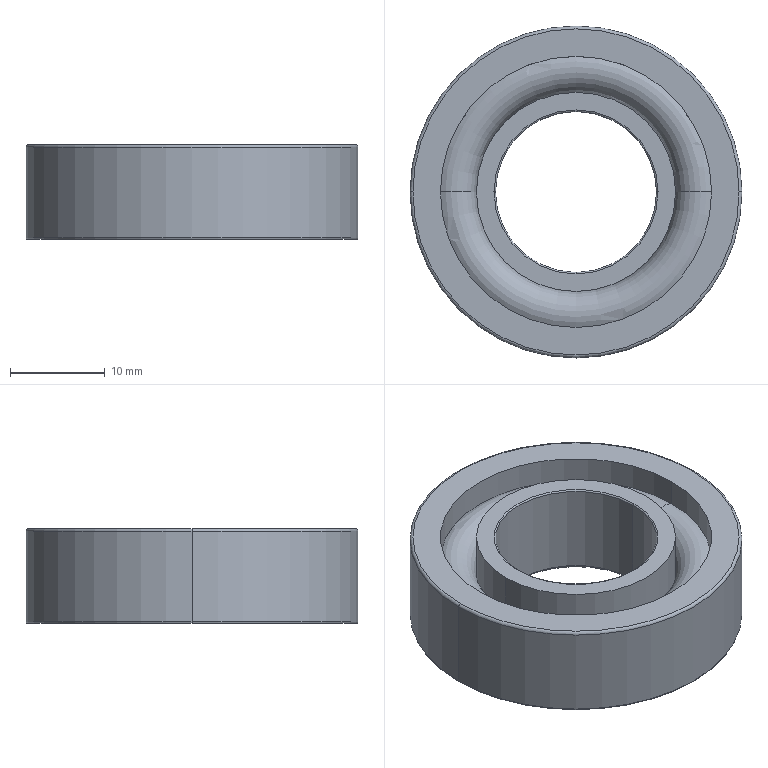Part | SolidWorks | features BaseBody 1 | 1 solid | 28 faces | box 35 x 35 x 10 mm | volume 5588 mm3 | torus 12 | cylinder 12 | plane 4 | commonest cylinder face diameters 17 x2 21 x2 23.75 x2 28.6 x2 31 x2 35 x2
STEP:
#1=CARTESIAN_POINT('',(-17.5,0.,-9.85));
#2=VERTEX_POINT('',#1);
#3=CARTESIAN_POINT('',(17.5,0.,-9.85));
#4=VERTEX_POINT('',#3);
#5=CARTESIAN_POINT('',(0.,0.,-9.85));
#6=DIRECTION('',(0.,0.,-1.));
#7=DIRECTION('',(-1.,0.,0.));
#8=AXIS2_PLACEMENT_3D('',#5,#6,#7);
#9=CIRCLE('',#8,17.5);
#10=EDGE_CURVE('',#2,#4,#9,.T.);
#11=ORIENTED_EDGE('',*,*,#10,.T.);
#12=CARTESIAN_POINT('',(17.35,0.,-10.));
#13=VERTEX_POINT('',#12);
#14=CARTESIAN_POINT('',(17.35,0.,-9.85));
#15=DIRECTION('',(0.,1.,0.));
#16=DIRECTION('',(-1.,0.,0.));
#17=AXIS2_PLACEMENT_3D('',#14,#15,#16);
#18=CIRCLE('',#17,0.15);
#19=EDGE_CURVE('',#4,#13,#18,.T.);
#20=ORIENTED_EDGE('',*,*,#19,.T.);
#21=CARTESIAN_POINT('',(-17.35,0.,-10.));
#22=VERTEX_POINT('',#21);
#23=CARTESIAN_POINT('',(0.,0.,-10.));
#24=DIRECTION('',(0.,0.,-1.));
#25=DIRECTION('',(-1.,0.,0.));
#26=AXIS2_PLACEMENT_3D('',#23,#24,#25);
#27=CIRCLE('',#26,17.35);
#28=EDGE_CURVE('',#22,#13,#27,.T.);
#29=ORIENTED_EDGE('',*,*,#28,.F.);
#30=CARTESIAN_POINT('',(-17.35,0.,-9.85));
#31=DIRECTION('',(0.,-1.,0.));
#32=DIRECTION('',(0.,0.,-1.));
#33=AXIS2_PLACEMENT_3D('',#30,#31,#32);
#34=CIRCLE('',#33,0.15);
#35=EDGE_CURVE('',#2,#22,#34,.T.);
#36=ORIENTED_EDGE('',*,*,#35,.F.);
#37=EDGE_LOOP('',(#11,#20,#29,#36));
#38=FACE_OUTER_BOUND('',#37,.T.);
#39=CARTESIAN_POINT('',(0.,0.,-9.85));
#40=DIRECTION('',(0.,0.,-1.));
#41=DIRECTION('',(-1.,0.,0.));
#42=AXIS2_PLACEMENT_3D('',#39,#40,#41);
#43=TOROIDAL_SURFACE('',#42,17.35,0.15);
#44=ADVANCED_FACE('',(#38),#43,.T.);
#45=CARTESIAN_POINT('',(15.5,0.,-5.));
#46=VERTEX_POINT('',#45);
#47=CARTESIAN_POINT('',(-15.5,0.,-5.));
#48=VERTEX_POINT('',#47);
#49=CARTESIAN_POINT('',(0.,0.,-5.));
#50=DIRECTION('',(0.,0.,-1.));
#51=DIRECTION('',(-1.,0.,0.));
#52=AXIS2_PLACEMENT_3D('',#49,#50,#51);
#53=CIRCLE('',#52,15.5);
#54=EDGE_CURVE('',#46,#48,#53,.T.);
#55=ORIENTED_EDGE('',*,*,#54,.F.);
#56=CARTESIAN_POINT('',(15.5,0.,-10.));
#57=VERTEX_POINT('',#56);
#58=CARTESIAN_POINT('',(15.5,0.,-10.));
#59=DIRECTION('',(0.,0.,-1.));
#60=VECTOR('',#59,1000.);
#61=LINE('',#58,#60);
#62=EDGE_CURVE('',#46,#57,#61,.T.);
#63=ORIENTED_EDGE('',*,*,#62,.T.);
#64=CARTESIAN_POINT('',(-15.5,0.,-10.));
#65=VERTEX_POINT('',#64);
#66=CARTESIAN_POINT('',(0.,0.,-10.));
#67=DIRECTION('',(0.,0.,-1.));
#68=DIRECTION('',(-1.,0.,0.));
#69=AXIS2_PLACEMENT_3D('',#66,#67,#68);
#70=CIRCLE('',#69,15.5);
#71=EDGE_CURVE('',#57,#65,#70,.T.);
#72=ORIENTED_EDGE('',*,*,#71,.T.);
#73=CARTESIAN_POINT('',(-15.5,0.,-10.));
#74=DIRECTION('',(0.,0.,-1.));
#75=VECTOR('',#74,1000.);
#76=LINE('',#73,#75);
#77=EDGE_CURVE('',#48,#65,#76,.T.);
#78=ORIENTED_EDGE('',*,*,#77,.F.);
#79=EDGE_LOOP('',(#55,#63,#72,#78));
#80=FACE_OUTER_BOUND('',#79,.T.);
#81=CARTESIAN_POINT('',(0.,0.,-10.));
#82=DIRECTION('',(0.,0.,-1.));
#83=DIRECTION('',(-1.,0.,0.));
#84=AXIS2_PLACEMENT_3D('',#81,#82,#83);
#85=CYLINDRICAL_SURFACE('',#84,15.5);
#86=ADVANCED_FACE('',(#80),#85,.F.);
#87=CARTESIAN_POINT('',(-17.5,0.,-0.3));
#88=VERTEX_POINT('',#87);
#89=CARTESIAN_POINT('',(17.5,0.,-0.3));
#90=VERTEX_POINT('',#89);
#91=CARTESIAN_POINT('',(0.,0.,-0.3));
#92=DIRECTION('',(0.,0.,-1.));
#93=DIRECTION('',(-1.,0.,0.));
#94=AXIS2_PLACEMENT_3D('',#91,#92,#93);
#95=CIRCLE('',#94,17.5);
#96=EDGE_CURVE('',#88,#90,#95,.T.);
#97=ORIENTED_EDGE('',*,*,#96,.T.);
#98=CARTESIAN_POINT('',(17.5,0.,-10.));
#99=DIRECTION('',(0.,0.,-1.));
#100=VECTOR('',#99,1000.);
#101=LINE('',#98,#100);
#102=EDGE_CURVE('',#90,#4,#101,.T.);
#103=ORIENTED_EDGE('',*,*,#102,.T.);
#104=ORIENTED_EDGE('',*,*,#10,.F.);
#105=CARTESIAN_POINT('',(-17.5,0.,-10.));
#106=DIRECTION('',(0.,0.,-1.));
#107=VECTOR('',#106,1000.);
#108=LINE('',#105,#107);
#109=EDGE_CURVE('',#88,#2,#108,.T.);
#110=ORIENTED_EDGE('',*,*,#109,.F.);
#111=EDGE_LOOP('',(#97,#103,#104,#110));
#112=FACE_OUTER_BOUND('',#111,.T.);
#113=CARTESIAN_POINT('',(0.,0.,-10.));
#114=DIRECTION('',(0.,0.,-1.));
#115=DIRECTION('',(-1.,0.,0.));
#116=AXIS2_PLACEMENT_3D('',#113,#114,#115);
#117=CYLINDRICAL_SURFACE('',#116,17.5);
#118=ADVANCED_FACE('',(#112),#117,.T.);
#119=CARTESIAN_POINT('',(0.,0.,-5.));
#120=DIRECTION('',(0.,0.,-1.));
#121=DIRECTION('',(-1.,0.,0.));
#122=AXIS2_PLACEMENT_3D('',#119,#120,#121);
#123=CIRCLE('',#122,15.5);
#124=EDGE_CURVE('',#48,#46,#123,.T.);
#125=ORIENTED_EDGE('',*,*,#124,.T.);
#126=CARTESIAN_POINT('',(11.875,0.,-7.233));
#127=VERTEX_POINT('',#126);
#128=CARTESIAN_POINT('',(13.,0.,-5.));
#129=DIRECTION('',(0.,1.,0.));
#130=DIRECTION('',(-1.,0.,0.));
#131=AXIS2_PLACEMENT_3D('',#128,#129,#130);
#132=CIRCLE('',#131,2.5);
#133=EDGE_CURVE('',#46,#127,#132,.T.);
#134=ORIENTED_EDGE('',*,*,#133,.T.);
#135=CARTESIAN_POINT('',(-11.875,0.,-7.233));
#136=VERTEX_POINT('',#135);
#137=CARTESIAN_POINT('',(0.,0.,-7.233));
#138=DIRECTION('',(0.,0.,-1.));
#139=DIRECTION('',(-1.,0.,0.));
#140=AXIS2_PLACEMENT_3D('',#137,#138,#139);
#141=CIRCLE('',#140,11.875);
#142=EDGE_CURVE('',#136,#127,#141,.T.);
#143=ORIENTED_EDGE('',*,*,#142,.F.);
#144=CARTESIAN_POINT('',(-13.,0.,-5.));
#145=DIRECTION('',(0.,-1.,0.));
#146=DIRECTION('',(0.,0.,-1.));
#147=AXIS2_PLACEMENT_3D('',#144,#145,#146);
#148=CIRCLE('',#147,2.5);
#149=EDGE_CURVE('',#48,#136,#148,.T.);
#150=ORIENTED_EDGE('',*,*,#149,.F.);
#151=EDGE_LOOP('',(#125,#134,#143,#150));
#152=FACE_OUTER_BOUND('',#151,.T.);
#153=CARTESIAN_POINT('',(0.,0.,-5.));
#154=DIRECTION('',(0.,0.,-1.));
#155=DIRECTION('',(-1.,0.,0.));
#156=AXIS2_PLACEMENT_3D('',#153,#154,#155);
#157=TOROIDAL_SURFACE('',#156,13.,2.5);
#158=ADVANCED_FACE('',(#152),#157,.T.);
#159=CARTESIAN_POINT('',(-17.2,0.,0.));
#160=VERTEX_POINT('',#159);
#161=CARTESIAN_POINT('',(17.2,0.,0.));
#162=VERTEX_POINT('',#161);
#163=CARTESIAN_POINT('',(0.,0.,0.));
#164=DIRECTION('',(0.,0.,-1.));
#165=DIRECTION('',(-1.,0.,0.));
#166=AXIS2_PLACEMENT_3D('',#163,#164,#165);
#167=CIRCLE('',#166,17.2);
#168=EDGE_CURVE('',#160,#162,#167,.T.);
#169=ORIENTED_EDGE('',*,*,#168,.T.);
#170=CARTESIAN_POINT('',(17.2,0.,-0.3));
#171=DIRECTION('',(0.,1.,0.));
#172=DIRECTION('',(-1.,0.,0.));
#173=AXIS2_PLACEMENT_3D('',#170,#171,#172);
#174=CIRCLE('',#173,0.3);
#175=EDGE_CURVE('',#162,#90,#174,.T.);
#176=ORIENTED_EDGE('',*,*,#175,.T.);
#177=ORIENTED_EDGE('',*,*,#96,.F.);
#178=CARTESIAN_POINT('',(-17.2,0.,-0.3));
#179=DIRECTION('',(0.,-1.,0.));
#180=DIRECTION('',(0.,0.,-1.));
#181=AXIS2_PLACEMENT_3D('',#178,#179,#180);
#182=CIRCLE('',#181,0.3);
#183=EDGE_CURVE('',#160,#88,#182,.T.);
#184=ORIENTED_EDGE('',*,*,#183,.F.);
#185=EDGE_LOOP('',(#169,#176,#177,#184));
#186=FACE_OUTER_BOUND('',#185,.T.);
#187=CARTESIAN_POINT('',(0.,0.,-0.3));
#188=DIRECTION('',(0.,0.,-1.));
#189=DIRECTION('',(-1.,0.,0.));
#190=AXIS2_PLACEMENT_3D('',#187,#188,#189);
#191=TOROIDAL_SURFACE('',#190,17.2,0.3);
#192=ADVANCED_FACE('',(#186),#191,.T.);
#193=ORIENTED_EDGE('',*,*,#142,.T.);
#194=CARTESIAN_POINT('',(11.875,0.,-10.));
#195=VERTEX_POINT('',#194);
#196=CARTESIAN_POINT('',(11.875,0.,-10.));
#197=DIRECTION('',(0.,0.,-1.));
#198=VECTOR('',#197,1000.);
#199=LINE('',#196,#198);
#200=EDGE_CURVE('',#127,#195,#199,.T.);
#201=ORIENTED_EDGE('',*,*,#200,.T.);
#202=CARTESIAN_POINT('',(-11.875,0.,-10.));
#203=VERTEX_POINT('',#202);
#204=CARTESIAN_POINT('',(0.,0.,-10.));
#205=DIRECTION('',(0.,0.,-1.));
#206=DIRECTION('',(-1.,0.,0.));
#207=AXIS2_PLACEMENT_3D('',#204,#205,#206);
#208=CIRCLE('',#207,11.875);
#209=EDGE_CURVE('',#203,#195,#208,.T.);
#210=ORIENTED_EDGE('',*,*,#209,.F.);
#211=CARTESIAN_POINT('',(-11.875,0.,-10.));
#212=DIRECTION('',(0.,0.,-1.));
#213=VECTOR('',#212,1000.);
#214=LINE('',#211,#213);
#215=EDGE_CURVE('',#136,#203,#214,.T.);
#216=ORIENTED_EDGE('',*,*,#215,.F.);
#217=EDGE_LOOP('',(#193,#201,#210,#216));
#218=FACE_OUTER_BOUND('',#217,.T.);
#219=CARTESIAN_POINT('',(0.,0.,-10.));
#220=DIRECTION('',(0.,0.,-1.));
#221=DIRECTION('',(-1.,0.,0.));
#222=AXIS2_PLACEMENT_3D('',#219,#220,#221);
#223=CYLINDRICAL_SURFACE('',#222,11.875);
#224=ADVANCED_FACE('',(#218),#223,.T.);
#225=CARTESIAN_POINT('',(14.3,0.,0.));
#226=VERTEX_POINT('',#225);
#227=CARTESIAN_POINT('',(-14.3,0.,0.));
#228=VERTEX_POINT('',#227);
#229=CARTESIAN_POINT('',(0.,0.,0.));
#230=DIRECTION('',(0.,0.,-1.));
#231=DIRECTION('',(-1.,0.,0.));
#232=AXIS2_PLACEMENT_3D('',#229,#230,#231);
#233=CIRCLE('',#232,14.3);
#234=EDGE_CURVE('',#226,#228,#233,.T.);
#235=ORIENTED_EDGE('',*,*,#234,.F.);
#236=CARTESIAN_POINT('',(14.3,0.,-2.865));
#237=VERTEX_POINT('',#236);
#238=CARTESIAN_POINT('',(14.3,0.,-10.));
#239=DIRECTION('',(0.,0.,-1.));
#240=VECTOR('',#239,1000.);
#241=LINE('',#238,#240);
#242=EDGE_CURVE('',#226,#237,#241,.T.);
#243=ORIENTED_EDGE('',*,*,#242,.T.);
#244=CARTESIAN_POINT('',(-14.3,0.,-2.865));
#245=VERTEX_POINT('',#244);
#246=CARTESIAN_POINT('',(0.,0.,-2.865));
#247=DIRECTION('',(0.,0.,-1.));
#248=DIRECTION('',(-1.,0.,0.));
#249=AXIS2_PLACEMENT_3D('',#246,#247,#248);
#250=CIRCLE('',#249,14.3);
#251=EDGE_CURVE('',#237,#245,#250,.T.);
#252=ORIENTED_EDGE('',*,*,#251,.T.);
#253=CARTESIAN_POINT('',(-14.3,0.,-10.));
#254=DIRECTION('',(0.,0.,-1.));
#255=VECTOR('',#254,1000.);
#256=LINE('',#253,#255);
#257=EDGE_CURVE('',#228,#245,#256,.T.);
#258=ORIENTED_EDGE('',*,*,#257,.F.);
#259=EDGE_LOOP('',(#235,#243,#252,#258));
#260=FACE_OUTER_BOUND('',#259,.T.);
#261=CARTESIAN_POINT('',(0.,0.,-10.));
#262=DIRECTION('',(0.,0.,-1.));
#263=DIRECTION('',(-1.,0.,0.));
#264=AXIS2_PLACEMENT_3D('',#261,#262,#263);
#265=CYLINDRICAL_SURFACE('',#264,14.3);
#266=ADVANCED_FACE('',(#260),#265,.F.);
#267=CARTESIAN_POINT('',(-8.8,0.,-10.));
#268=VERTEX_POINT('',#267);
#269=CARTESIAN_POINT('',(8.8,0.,-10.));
#270=VERTEX_POINT('',#269);
#271=CARTESIAN_POINT('',(0.,0.,-10.));
#272=DIRECTION('',(0.,0.,-1.));
#273=DIRECTION('',(-1.,0.,0.));
#274=AXIS2_PLACEMENT_3D('',#271,#272,#273);
#275=CIRCLE('',#274,8.8);
#276=EDGE_CURVE('',#268,#270,#275,.T.);
#277=ORIENTED_EDGE('',*,*,#276,.T.);
#278=CARTESIAN_POINT('',(8.5,0.,-9.7));
#279=VERTEX_POINT('',#278);
#280=CARTESIAN_POINT('',(8.8,0.,-9.7));
#281=DIRECTION('',(0.,1.,0.));
#282=DIRECTION('',(-1.,0.,0.));
#283=AXIS2_PLACEMENT_3D('',#280,#281,#282);
#284=CIRCLE('',#283,0.3);
#285=EDGE_CURVE('',#270,#279,#284,.T.);
#286=ORIENTED_EDGE('',*,*,#285,.T.);
#287=CARTESIAN_POINT('',(-8.5,0.,-9.7));
#288=VERTEX_POINT('',#287);
#289=CARTESIAN_POINT('',(0.,0.,-9.7));
#290=DIRECTION('',(0.,0.,-1.));
#291=DIRECTION('',(-1.,0.,0.));
#292=AXIS2_PLACEMENT_3D('',#289,#290,#291);
#293=CIRCLE('',#292,8.5);
#294=EDGE_CURVE('',#288,#279,#293,.T.);
#295=ORIENTED_EDGE('',*,*,#294,.F.);
#296=CARTESIAN_POINT('',(-8.8,0.,-9.7));
#297=DIRECTION('',(0.,-1.,0.));
#298=DIRECTION('',(0.,0.,-1.));
#299=AXIS2_PLACEMENT_3D('',#296,#297,#298);
#300=CIRCLE('',#299,0.3);
#301=EDGE_CURVE('',#268,#288,#300,.T.);
#302=ORIENTED_EDGE('',*,*,#301,.F.);
#303=EDGE_LOOP('',(#277,#286,#295,#302));
#304=FACE_OUTER_BOUND('',#303,.T.);
#305=CARTESIAN_POINT('',(0.,0.,-9.7));
#306=DIRECTION('',(0.,0.,-1.));
#307=DIRECTION('',(-1.,0.,0.));
#308=AXIS2_PLACEMENT_3D('',#305,#306,#307);
#309=TOROIDAL_SURFACE('',#308,8.8,0.3);
#310=ADVANCED_FACE('',(#304),#309,.T.);
#311=CARTESIAN_POINT('',(-10.5,0.,-5.));
#312=VERTEX_POINT('',#311);
#313=CARTESIAN_POINT('',(10.5,0.,-5.));
#314=VERTEX_POINT('',#313);
#315=CARTESIAN_POINT('',(0.,0.,-5.));
#316=DIRECTION('',(0.,0.,-1.));
#317=DIRECTION('',(-1.,0.,0.));
#318=AXIS2_PLACEMENT_3D('',#315,#316,#317);
#319=CIRCLE('',#318,10.5);
#320=EDGE_CURVE('',#312,#314,#319,.T.);
#321=ORIENTED_EDGE('',*,*,#320,.T.);
#322=CARTESIAN_POINT('',(13.,0.,-5.));
#323=DIRECTION('',(0.,1.,0.));
#324=DIRECTION('',(-1.,0.,0.));
#325=AXIS2_PLACEMENT_3D('',#322,#323,#324);
#326=CIRCLE('',#325,2.5);
#327=EDGE_CURVE('',#314,#237,#326,.T.);
#328=ORIENTED_EDGE('',*,*,#327,.T.);
#329=CARTESIAN_POINT('',(0.,0.,-2.865));
#330=DIRECTION('',(0.,0.,-1.));
#331=DIRECTION('',(-1.,0.,0.));
#332=AXIS2_PLACEMENT_3D('',#329,#330,#331);
#333=CIRCLE('',#332,14.3);
#334=EDGE_CURVE('',#245,#237,#333,.T.);
#335=ORIENTED_EDGE('',*,*,#334,.F.);
#336=CARTESIAN_POINT('',(-13.,0.,-5.));
#337=DIRECTION('',(0.,-1.,0.));
#338=DIRECTION('',(0.,0.,-1.));
#339=AXIS2_PLACEMENT_3D('',#336,#337,#338);
#340=CIRCLE('',#339,2.5);
#341=EDGE_CURVE('',#312,#245,#340,.T.);
#342=ORIENTED_EDGE('',*,*,#341,.F.);
#343=EDGE_LOOP('',(#321,#328,#335,#342));
#344=FACE_OUTER_BOUND('',#343,.T.);
#345=CARTESIAN_POINT('',(0.,0.,-5.));
#346=DIRECTION('',(0.,0.,-1.));
#347=DIRECTION('',(-1.,0.,0.));
#348=AXIS2_PLACEMENT_3D('',#345,#346,#347);
#349=TOROIDAL_SURFACE('',#348,13.,2.5);
#350=ADVANCED_FACE('',(#344),#349,.T.);
#351=CARTESIAN_POINT('',(8.5,0.,-0.15));
#352=VERTEX_POINT('',#351);
#353=CARTESIAN_POINT('',(-8.5,0.,-0.15));
#354=VERTEX_POINT('',#353);
#355=CARTESIAN_POINT('',(0.,0.,-0.15));
#356=DIRECTION('',(0.,0.,-1.));
#357=DIRECTION('',(-1.,0.,0.));
#358=AXIS2_PLACEMENT_3D('',#355,#356,#357);
#359=CIRCLE('',#358,8.5);
#360=EDGE_CURVE('',#352,#354,#359,.T.);
#361=ORIENTED_EDGE('',*,*,#360,.F.);
#362=CARTESIAN_POINT('',(8.5,0.,-10.));
#363=DIRECTION('',(0.,0.,-1.));
#364=VECTOR('',#363,1000.);
#365=LINE('',#362,#364);
#366=EDGE_CURVE('',#352,#279,#365,.T.);
#367=ORIENTED_EDGE('',*,*,#366,.T.);
#368=CARTESIAN_POINT('',(0.,0.,-9.7));
#369=DIRECTION('',(0.,0.,-1.));
#370=DIRECTION('',(-1.,0.,0.));
#371=AXIS2_PLACEMENT_3D('',#368,#369,#370);
#372=CIRCLE('',#371,8.5);
#373=EDGE_CURVE('',#279,#288,#372,.T.);
#374=ORIENTED_EDGE('',*,*,#373,.T.);
#375=CARTESIAN_POINT('',(-8.5,0.,-10.));
#376=DIRECTION('',(0.,0.,-1.));
#377=VECTOR('',#376,1000.);
#378=LINE('',#375,#377);
#379=EDGE_CURVE('',#354,#288,#378,.T.);
#380=ORIENTED_EDGE('',*,*,#379,.F.);
#381=EDGE_LOOP('',(#361,#367,#374,#380));
#382=FACE_OUTER_BOUND('',#381,.T.);
#383=CARTESIAN_POINT('',(0.,0.,-10.));
#384=DIRECTION('',(0.,0.,-1.));
#385=DIRECTION('',(-1.,0.,0.));
#386=AXIS2_PLACEMENT_3D('',#383,#384,#385);
#387=CYLINDRICAL_SURFACE('',#386,8.5);
#388=ADVANCED_FACE('',(#382),#387,.F.);
#389=CARTESIAN_POINT('',(-10.5,0.,0.));
#390=VERTEX_POINT('',#389);
#391=CARTESIAN_POINT('',(10.5,0.,0.));
#392=VERTEX_POINT('',#391);
#393=CARTESIAN_POINT('',(0.,0.,0.));
#394=DIRECTION('',(0.,0.,-1.));
#395=DIRECTION('',(-1.,0.,0.));
#396=AXIS2_PLACEMENT_3D('',#393,#394,#395);
#397=CIRCLE('',#396,10.5);
#398=EDGE_CURVE('',#390,#392,#397,.T.);
#399=ORIENTED_EDGE('',*,*,#398,.T.);
#400=CARTESIAN_POINT('',(10.5,0.,-10.));
#401=DIRECTION('',(0.,0.,-1.));
#402=VECTOR('',#401,1000.);
#403=LINE('',#400,#402);
#404=EDGE_CURVE('',#392,#314,#403,.T.);
#405=ORIENTED_EDGE('',*,*,#404,.T.);
#406=ORIENTED_EDGE('',*,*,#320,.F.);
#407=CARTESIAN_POINT('',(-10.5,0.,-10.));
#408=DIRECTION('',(0.,0.,-1.));
#409=VECTOR('',#408,1000.);
#410=LINE('',#407,#409);
#411=EDGE_CURVE('',#390,#312,#410,.T.);
#412=ORIENTED_EDGE('',*,*,#411,.F.);
#413=EDGE_LOOP('',(#399,#405,#406,#412));
#414=FACE_OUTER_BOUND('',#413,.T.);
#415=CARTESIAN_POINT('',(0.,0.,-10.));
#416=DIRECTION('',(0.,0.,-1.));
#417=DIRECTION('',(-1.,0.,0.));
#418=AXIS2_PLACEMENT_3D('',#415,#416,#417);
#419=CYLINDRICAL_SURFACE('',#418,10.5);
#420=ADVANCED_FACE('',(#414),#419,.T.);
#421=CARTESIAN_POINT('',(0.,0.,-0.15));
#422=DIRECTION('',(0.,0.,-1.));
#423=DIRECTION('',(-1.,0.,0.));
#424=AXIS2_PLACEMENT_3D('',#421,#422,#423);
#425=CIRCLE('',#424,8.5);
#426=EDGE_CURVE('',#354,#352,#425,.T.);
#427=ORIENTED_EDGE('',*,*,#426,.T.);
#428=CARTESIAN_POINT('',(8.65,0.,0.));
#429=VERTEX_POINT('',#428);
#430=CARTESIAN_POINT('',(8.65,0.,-0.15));
#431=DIRECTION('',(0.,1.,0.));
#432=DIRECTION('',(-1.,0.,0.));
#433=AXIS2_PLACEMENT_3D('',#430,#431,#432);
#434=CIRCLE('',#433,0.15);
#435=EDGE_CURVE('',#352,#429,#434,.T.);
#436=ORIENTED_EDGE('',*,*,#435,.T.);
#437=CARTESIAN_POINT('',(-8.65,0.,0.));
#438=VERTEX_POINT('',#437);
#439=CARTESIAN_POINT('',(0.,0.,0.));
#440=DIRECTION('',(0.,0.,-1.));
#441=DIRECTION('',(-1.,0.,0.));
#442=AXIS2_PLACEMENT_3D('',#439,#440,#441);
#443=CIRCLE('',#442,8.65);
#444=EDGE_CURVE('',#438,#429,#443,.T.);
#445=ORIENTED_EDGE('',*,*,#444,.F.);
#446=CARTESIAN_POINT('',(-8.65,0.,-0.15));
#447=DIRECTION('',(0.,-1.,0.));
#448=DIRECTION('',(0.,0.,-1.));
#449=AXIS2_PLACEMENT_3D('',#446,#447,#448);
#450=CIRCLE('',#449,0.15);
#451=EDGE_CURVE('',#354,#438,#450,.T.);
#452=ORIENTED_EDGE('',*,*,#451,.F.);
#453=EDGE_LOOP('',(#427,#436,#445,#452));
#454=FACE_OUTER_BOUND('',#453,.T.);
#455=CARTESIAN_POINT('',(0.,0.,-0.15));
#456=DIRECTION('',(0.,0.,-1.));
#457=DIRECTION('',(-1.,0.,0.));
#458=AXIS2_PLACEMENT_3D('',#455,#456,#457);
#459=TOROIDAL_SURFACE('',#458,8.65,0.15);
#460=ADVANCED_FACE('',(#454),#459,.T.);
#461=ORIENTED_EDGE('',*,*,#444,.T.);
#462=CARTESIAN_POINT('',(0.,0.,0.));
#463=DIRECTION('',(0.,0.,-1.));
#464=DIRECTION('',(-1.,0.,0.));
#465=AXIS2_PLACEMENT_3D('',#462,#463,#464);
#466=CIRCLE('',#465,8.65);
#467=EDGE_CURVE('',#429,#438,#466,.T.);
#468=ORIENTED_EDGE('',*,*,#467,.T.);
#469=EDGE_LOOP('',(#461,#468));
#470=FACE_BOUND('',#469,.T.);
#471=ORIENTED_EDGE('',*,*,#398,.F.);
#472=CARTESIAN_POINT('',(0.,0.,0.));
#473=DIRECTION('',(0.,0.,-1.));
#474=DIRECTION('',(-1.,0.,0.));
#475=AXIS2_PLACEMENT_3D('',#472,#473,#474);
#476=CIRCLE('',#475,10.5);
#477=EDGE_CURVE('',#392,#390,#476,.T.);
#478=ORIENTED_EDGE('',*,*,#477,.F.);
#479=EDGE_LOOP('',(#471,#478));
#480=FACE_OUTER_BOUND('',#479,.T.);
#481=CARTESIAN_POINT('',(0.,10.5,0.));
#482=DIRECTION('',(0.,0.,1.));
#483=DIRECTION('',(1.,0.,0.));
#484=AXIS2_PLACEMENT_3D('',#481,#482,#483);
#485=PLANE('',#484);
#486=ADVANCED_FACE('',(#470,#480),#485,.T.);
#487=ORIENTED_EDGE('',*,*,#435,.F.);
#488=ORIENTED_EDGE('',*,*,#360,.T.);
#489=ORIENTED_EDGE('',*,*,#451,.T.);
#490=ORIENTED_EDGE('',*,*,#467,.F.);
#491=EDGE_LOOP('',(#487,#488,#489,#490));
#492=FACE_OUTER_BOUND('',#491,.T.);
#493=CARTESIAN_POINT('',(0.,0.,-0.15));
#494=DIRECTION('',(0.,0.,-1.));
#495=DIRECTION('',(-1.,0.,0.));
#496=AXIS2_PLACEMENT_3D('',#493,#494,#495);
#497=TOROIDAL_SURFACE('',#496,8.65,0.15);
#498=ADVANCED_FACE('',(#492),#497,.T.);
#499=ORIENTED_EDGE('',*,*,#404,.F.);
#500=ORIENTED_EDGE('',*,*,#477,.T.);
#501=ORIENTED_EDGE('',*,*,#411,.T.);
#502=CARTESIAN_POINT('',(0.,0.,-5.));
#503=DIRECTION('',(0.,0.,-1.));
#504=DIRECTION('',(-1.,0.,0.));
#505=AXIS2_PLACEMENT_3D('',#502,#503,#504);
#506=CIRCLE('',#505,10.5);
#507=EDGE_CURVE('',#314,#312,#506,.T.);
#508=ORIENTED_EDGE('',*,*,#507,.F.);
#509=EDGE_LOOP('',(#499,#500,#501,#508));
#510=FACE_OUTER_BOUND('',#509,.T.);
#511=CARTESIAN_POINT('',(0.,0.,-10.));
#512=DIRECTION('',(0.,0.,-1.));
#513=DIRECTION('',(-1.,0.,0.));
#514=AXIS2_PLACEMENT_3D('',#511,#512,#513);
#515=CYLINDRICAL_SURFACE('',#514,10.5);
#516=ADVANCED_FACE('',(#510),#515,.T.);
#517=ORIENTED_EDGE('',*,*,#366,.F.);
#518=ORIENTED_EDGE('',*,*,#426,.F.);
#519=ORIENTED_EDGE('',*,*,#379,.T.);
#520=ORIENTED_EDGE('',*,*,#294,.T.);
#521=EDGE_LOOP('',(#517,#518,#519,#520));
#522=FACE_OUTER_BOUND('',#521,.T.);
#523=CARTESIAN_POINT('',(0.,0.,-10.));
#524=DIRECTION('',(0.,0.,-1.));
#525=DIRECTION('',(-1.,0.,0.));
#526=AXIS2_PLACEMENT_3D('',#523,#524,#525);
#527=CYLINDRICAL_SURFACE('',#526,8.5);
#528=ADVANCED_FACE('',(#522),#527,.F.);
#529=ORIENTED_EDGE('',*,*,#327,.F.);
#530=ORIENTED_EDGE('',*,*,#507,.T.);
#531=ORIENTED_EDGE('',*,*,#341,.T.);
#532=ORIENTED_EDGE('',*,*,#251,.F.);
#533=EDGE_LOOP('',(#529,#530,#531,#532));
#534=FACE_OUTER_BOUND('',#533,.T.);
#535=CARTESIAN_POINT('',(0.,0.,-5.));
#536=DIRECTION('',(0.,0.,-1.));
#537=DIRECTION('',(-1.,0.,0.));
#538=AXIS2_PLACEMENT_3D('',#535,#536,#537);
#539=TOROIDAL_SURFACE('',#538,13.,2.5);
#540=ADVANCED_FACE('',(#534),#539,.T.);
#541=ORIENTED_EDGE('',*,*,#285,.F.);
#542=CARTESIAN_POINT('',(0.,0.,-10.));
#543=DIRECTION('',(0.,0.,-1.));
#544=DIRECTION('',(-1.,0.,0.));
#545=AXIS2_PLACEMENT_3D('',#542,#543,#544);
#546=CIRCLE('',#545,8.8);
#547=EDGE_CURVE('',#270,#268,#546,.T.);
#548=ORIENTED_EDGE('',*,*,#547,.T.);
#549=ORIENTED_EDGE('',*,*,#301,.T.);
#550=ORIENTED_EDGE('',*,*,#373,.F.);
#551=EDGE_LOOP('',(#541,#548,#549,#550));
#552=FACE_OUTER_BOUND('',#551,.T.);
#553=CARTESIAN_POINT('',(0.,0.,-9.7));
#554=DIRECTION('',(0.,0.,-1.));
#555=DIRECTION('',(-1.,0.,0.));
#556=AXIS2_PLACEMENT_3D('',#553,#554,#555);
#557=TOROIDAL_SURFACE('',#556,8.8,0.3);
#558=ADVANCED_FACE('',(#552),#557,.T.);
#559=ORIENTED_EDGE('',*,*,#242,.F.);
#560=CARTESIAN_POINT('',(0.,0.,0.));
#561=DIRECTION('',(0.,0.,-1.));
#562=DIRECTION('',(-1.,0.,0.));
#563=AXIS2_PLACEMENT_3D('',#560,#561,#562);
#564=CIRCLE('',#563,14.3);
#565=EDGE_CURVE('',#228,#226,#564,.T.);
#566=ORIENTED_EDGE('',*,*,#565,.F.);
#567=ORIENTED_EDGE('',*,*,#257,.T.);
#568=ORIENTED_EDGE('',*,*,#334,.T.);
#569=EDGE_LOOP('',(#559,#566,#567,#568));
#570=FACE_OUTER_BOUND('',#569,.T.);
#571=CARTESIAN_POINT('',(0.,0.,-10.));
#572=DIRECTION('',(0.,0.,-1.));
#573=DIRECTION('',(-1.,0.,0.));
#574=AXIS2_PLACEMENT_3D('',#571,#572,#573);
#575=CYLINDRICAL_SURFACE('',#574,14.3);
#576=ADVANCED_FACE('',(#570),#575,.F.);
#577=ORIENTED_EDGE('',*,*,#209,.T.);
#578=CARTESIAN_POINT('',(0.,0.,-10.));
#579=DIRECTION('',(0.,0.,-1.));
#580=DIRECTION('',(-1.,0.,0.));
#581=AXIS2_PLACEMENT_3D('',#578,#579,#580);
#582=CIRCLE('',#581,11.875);
#583=EDGE_CURVE('',#195,#203,#582,.T.);
#584=ORIENTED_EDGE('',*,*,#583,.T.);
#585=EDGE_LOOP('',(#577,#584));
#586=FACE_OUTER_BOUND('',#585,.T.);
#587=ORIENTED_EDGE('',*,*,#276,.F.);
#588=ORIENTED_EDGE('',*,*,#547,.F.);
#589=EDGE_LOOP('',(#587,#588));
#590=FACE_BOUND('',#589,.T.);
#591=CARTESIAN_POINT('',(0.,8.8,-10.));
#592=DIRECTION('',(0.,0.,-1.));
#593=DIRECTION('',(-1.,0.,0.));
#594=AXIS2_PLACEMENT_3D('',#591,#592,#593);
#595=PLANE('',#594);
#596=ADVANCED_FACE('',(#586,#590),#595,.T.);
#597=ORIENTED_EDGE('',*,*,#565,.T.);
#598=ORIENTED_EDGE('',*,*,#234,.T.);
#599=EDGE_LOOP('',(#597,#598));
#600=FACE_BOUND('',#599,.T.);
#601=ORIENTED_EDGE('',*,*,#168,.F.);
#602=CARTESIAN_POINT('',(0.,0.,0.));
#603=DIRECTION('',(0.,0.,-1.));
#604=DIRECTION('',(-1.,0.,0.));
#605=AXIS2_PLACEMENT_3D('',#602,#603,#604);
#606=CIRCLE('',#605,17.2);
#607=EDGE_CURVE('',#162,#160,#606,.T.);
#608=ORIENTED_EDGE('',*,*,#607,.F.);
#609=EDGE_LOOP('',(#601,#608));
#610=FACE_OUTER_BOUND('',#609,.T.);
#611=CARTESIAN_POINT('',(0.,17.2,0.));
#612=DIRECTION('',(0.,0.,1.));
#613=DIRECTION('',(1.,0.,0.));
#614=AXIS2_PLACEMENT_3D('',#611,#612,#613);
#615=PLANE('',#614);
#616=ADVANCED_FACE('',(#600,#610),#615,.T.);
#617=ORIENTED_EDGE('',*,*,#200,.F.);
#618=CARTESIAN_POINT('',(0.,0.,-7.233));
#619=DIRECTION('',(0.,0.,-1.));
#620=DIRECTION('',(-1.,0.,0.));
#621=AXIS2_PLACEMENT_3D('',#618,#619,#620);
#622=CIRCLE('',#621,11.875);
#623=EDGE_CURVE('',#127,#136,#622,.T.);
#624=ORIENTED_EDGE('',*,*,#623,.T.);
#625=ORIENTED_EDGE('',*,*,#215,.T.);
#626=ORIENTED_EDGE('',*,*,#583,.F.);
#627=EDGE_LOOP('',(#617,#624,#625,#626));
#628=FACE_OUTER_BOUND('',#627,.T.);
#629=CARTESIAN_POINT('',(0.,0.,-10.));
#630=DIRECTION('',(0.,0.,-1.));
#631=DIRECTION('',(-1.,0.,0.));
#632=AXIS2_PLACEMENT_3D('',#629,#630,#631);
#633=CYLINDRICAL_SURFACE('',#632,11.875);
#634=ADVANCED_FACE('',(#628),#633,.T.);
#635=ORIENTED_EDGE('',*,*,#175,.F.);
#636=ORIENTED_EDGE('',*,*,#607,.T.);
#637=ORIENTED_EDGE('',*,*,#183,.T.);
#638=CARTESIAN_POINT('',(0.,0.,-0.3));
#639=DIRECTION('',(0.,0.,-1.));
#640=DIRECTION('',(-1.,0.,0.));
#641=AXIS2_PLACEMENT_3D('',#638,#639,#640);
#642=CIRCLE('',#641,17.5);
#643=EDGE_CURVE('',#90,#88,#642,.T.);
#644=ORIENTED_EDGE('',*,*,#643,.F.);
#645=EDGE_LOOP('',(#635,#636,#637,#644));
#646=FACE_OUTER_BOUND('',#645,.T.);
#647=CARTESIAN_POINT('',(0.,0.,-0.3));
#648=DIRECTION('',(0.,0.,-1.));
#649=DIRECTION('',(-1.,0.,0.));
#650=AXIS2_PLACEMENT_3D('',#647,#648,#649);
#651=TOROIDAL_SURFACE('',#650,17.2,0.3);
#652=ADVANCED_FACE('',(#646),#651,.T.);
#653=ORIENTED_EDGE('',*,*,#133,.F.);
#654=ORIENTED_EDGE('',*,*,#54,.T.);
#655=ORIENTED_EDGE('',*,*,#149,.T.);
#656=ORIENTED_EDGE('',*,*,#623,.F.);
#657=EDGE_LOOP('',(#653,#654,#655,#656));
#658=FACE_OUTER_BOUND('',#657,.T.);
#659=CARTESIAN_POINT('',(0.,0.,-5.));
#660=DIRECTION('',(0.,0.,-1.));
#661=DIRECTION('',(-1.,0.,0.));
#662=AXIS2_PLACEMENT_3D('',#659,#660,#661);
#663=TOROIDAL_SURFACE('',#662,13.,2.5);
#664=ADVANCED_FACE('',(#658),#663,.T.);
#665=ORIENTED_EDGE('',*,*,#102,.F.);
#666=ORIENTED_EDGE('',*,*,#643,.T.);
#667=ORIENTED_EDGE('',*,*,#109,.T.);
#668=CARTESIAN_POINT('',(0.,0.,-9.85));
#669=DIRECTION('',(0.,0.,-1.));
#670=DIRECTION('',(-1.,0.,0.));
#671=AXIS2_PLACEMENT_3D('',#668,#669,#670);
#672=CIRCLE('',#671,17.5);
#673=EDGE_CURVE('',#4,#2,#672,.T.);
#674=ORIENTED_EDGE('',*,*,#673,.F.);
#675=EDGE_LOOP('',(#665,#666,#667,#674));
#676=FACE_OUTER_BOUND('',#675,.T.);
#677=CARTESIAN_POINT('',(0.,0.,-10.));
#678=DIRECTION('',(0.,0.,-1.));
#679=DIRECTION('',(-1.,0.,0.));
#680=AXIS2_PLACEMENT_3D('',#677,#678,#679);
#681=CYLINDRICAL_SURFACE('',#680,17.5);
#682=ADVANCED_FACE('',(#676),#681,.T.);
#683=ORIENTED_EDGE('',*,*,#62,.F.);
#684=ORIENTED_EDGE('',*,*,#124,.F.);
#685=ORIENTED_EDGE('',*,*,#77,.T.);
#686=CARTESIAN_POINT('',(0.,0.,-10.));
#687=DIRECTION('',(0.,0.,-1.));
#688=DIRECTION('',(-1.,0.,0.));
#689=AXIS2_PLACEMENT_3D('',#686,#687,#688);
#690=CIRCLE('',#689,15.5);
#691=EDGE_CURVE('',#65,#57,#690,.T.);
#692=ORIENTED_EDGE('',*,*,#691,.T.);
#693=EDGE_LOOP('',(#683,#684,#685,#692));
#694=FACE_OUTER_BOUND('',#693,.T.);
#695=CARTESIAN_POINT('',(0.,0.,-10.));
#696=DIRECTION('',(0.,0.,-1.));
#697=DIRECTION('',(-1.,0.,0.));
#698=AXIS2_PLACEMENT_3D('',#695,#696,#697);
#699=CYLINDRICAL_SURFACE('',#698,15.5);
#700=ADVANCED_FACE('',(#694),#699,.F.);
#701=ORIENTED_EDGE('',*,*,#19,.F.);
#702=ORIENTED_EDGE('',*,*,#673,.T.);
#703=ORIENTED_EDGE('',*,*,#35,.T.);
#704=CARTESIAN_POINT('',(0.,0.,-10.));
#705=DIRECTION('',(0.,0.,-1.));
#706=DIRECTION('',(-1.,0.,0.));
#707=AXIS2_PLACEMENT_3D('',#704,#705,#706);
#708=CIRCLE('',#707,17.35);
#709=EDGE_CURVE('',#13,#22,#708,.T.);
#710=ORIENTED_EDGE('',*,*,#709,.F.);
#711=EDGE_LOOP('',(#701,#702,#703,#710));
#712=FACE_OUTER_BOUND('',#711,.T.);
#713=CARTESIAN_POINT('',(0.,0.,-9.85));
#714=DIRECTION('',(0.,0.,-1.));
#715=DIRECTION('',(-1.,0.,0.));
#716=AXIS2_PLACEMENT_3D('',#713,#714,#715);
#717=TOROIDAL_SURFACE('',#716,17.35,0.15);
#718=ADVANCED_FACE('',(#712),#717,.T.);
#719=ORIENTED_EDGE('',*,*,#28,.T.);
#720=ORIENTED_EDGE('',*,*,#709,.T.);
#721=EDGE_LOOP('',(#719,#720));
#722=FACE_OUTER_BOUND('',#721,.T.);
#723=ORIENTED_EDGE('',*,*,#691,.F.);
#724=ORIENTED_EDGE('',*,*,#71,.F.);
#725=EDGE_LOOP('',(#723,#724));
#726=FACE_BOUND('',#725,.T.);
#727=CARTESIAN_POINT('',(0.,15.5,-10.));
#728=DIRECTION('',(0.,0.,-1.));
#729=DIRECTION('',(-1.,0.,0.));
#730=AXIS2_PLACEMENT_3D('',#727,#728,#729);
#731=PLANE('',#730);
#732=ADVANCED_FACE('',(#722,#726),#731,.T.);
#733=CLOSED_SHELL('',(#44,#86,#118,#158,#192,#224,#266,#310,#350,#388,#420,#460,#486,#498,#516,#528,#540,#558,#576,#596,#616,#634,#652,#664,#682,#700,#718,#732));
#734=MANIFOLD_SOLID_BREP('',#733);
#735=CARTESIAN_POINT('',(0.,0.,0.));
#736=DIRECTION('',(0.,0.,1.));
#737=DIRECTION('',(1.,0.,0.));
#738=AXIS2_PLACEMENT_3D('',#735,#736,#737);
#739=(LENGTH_UNIT()NAMED_UNIT(*)SI_UNIT(.MILLI.,.METRE.));
#740=UNCERTAINTY_MEASURE_WITH_UNIT(LENGTH_MEASURE(0.00001),#739,'','');
#741=(NAMED_UNIT(*)PLANE_ANGLE_UNIT()SI_UNIT($,.RADIAN.));
#742=(NAMED_UNIT(*)SI_UNIT($,.STERADIAN.)SOLID_ANGLE_UNIT());
#743=(GEOMETRIC_REPRESENTATION_CONTEXT(3)GLOBAL_UNCERTAINTY_ASSIGNED_CONTEXT((#740))GLOBAL_UNIT_ASSIGNED_CONTEXT((#739,#741,#742))REPRESENTATION_CONTEXT('',''));
#744=ADVANCED_BREP_SHAPE_REPRESENTATION('',(#734,#738),#743);